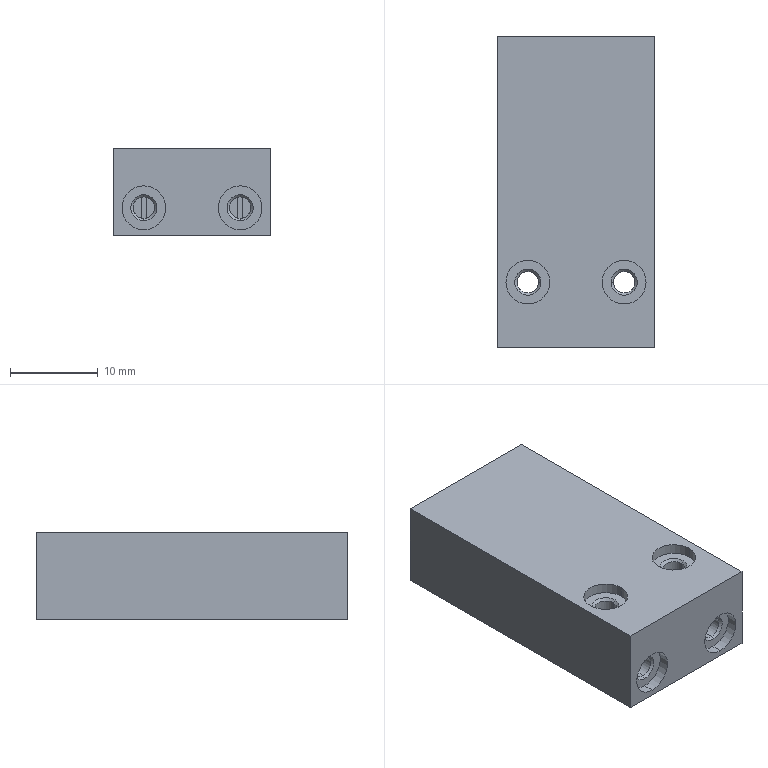Part | STEP file | 1 solid | 64 faces | box 18 x 35.6 x 10 mm | volume 6107 mm3 | cylinder 30 | plane 18 | cone 16 | commonest cylinder face diameters 2.459 x18 5 x12